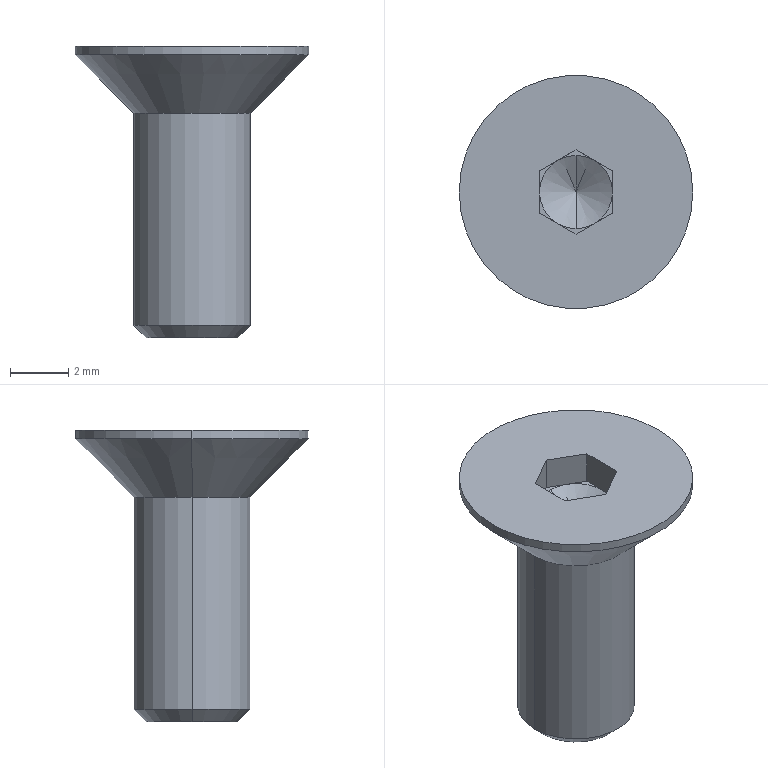Part | SolidWorks | features BaseBody 1 | 1 solid | 24 faces | box 8 x 8 x 10 mm | volume 162.002 mm3 | plane 14 | cone 6 | cylinder 4 | commonest cylinder face diameters 4 x2 8 x2
STEP:
#1=CARTESIAN_POINT('',(2.,0.,-7.271));
#2=VERTEX_POINT('',#1);
#3=CARTESIAN_POINT('',(-2.,0.,-7.271));
#4=VERTEX_POINT('',#3);
#5=CARTESIAN_POINT('',(0.,0.,-7.271));
#6=DIRECTION('',(0.,0.,1.));
#7=DIRECTION('',(1.,0.,0.));
#8=AXIS2_PLACEMENT_3D('',#5,#6,#7);
#9=CIRCLE('',#8,2.);
#10=EDGE_CURVE('',#2,#4,#9,.T.);
#11=ORIENTED_EDGE('',*,*,#10,.T.);
#12=CARTESIAN_POINT('',(-2.,0.,0.));
#13=VERTEX_POINT('',#12);
#14=CARTESIAN_POINT('',(-2.,0.,-7.7));
#15=DIRECTION('',(0.,0.,1.));
#16=VECTOR('',#15,1000.);
#17=LINE('',#14,#16);
#18=EDGE_CURVE('',#4,#13,#17,.T.);
#19=ORIENTED_EDGE('',*,*,#18,.T.);
#20=CARTESIAN_POINT('',(2.,0.,0.));
#21=VERTEX_POINT('',#20);
#22=CARTESIAN_POINT('',(0.,0.,0.));
#23=DIRECTION('',(0.,0.,-1.));
#24=DIRECTION('',(1.,0.,0.));
#25=AXIS2_PLACEMENT_3D('',#22,#23,#24);
#26=CIRCLE('',#25,2.);
#27=EDGE_CURVE('',#13,#21,#26,.T.);
#28=ORIENTED_EDGE('',*,*,#27,.T.);
#29=CARTESIAN_POINT('',(2.,0.,-7.7));
#30=DIRECTION('',(0.,0.,1.));
#31=VECTOR('',#30,1000.);
#32=LINE('',#29,#31);
#33=EDGE_CURVE('',#2,#21,#32,.T.);
#34=ORIENTED_EDGE('',*,*,#33,.F.);
#35=EDGE_LOOP('',(#11,#19,#28,#34));
#36=FACE_OUTER_BOUND('',#35,.T.);
#37=CARTESIAN_POINT('',(0.,0.,-7.7));
#38=DIRECTION('',(0.,0.,1.));
#39=DIRECTION('',(1.,0.,0.));
#40=AXIS2_PLACEMENT_3D('',#37,#38,#39);
#41=CYLINDRICAL_SURFACE('',#40,2.);
#42=ADVANCED_FACE('',(#36),#41,.T.);
#43=ORIENTED_EDGE('',*,*,#27,.F.);
#44=CARTESIAN_POINT('',(-4.,0.,2.));
#45=VERTEX_POINT('',#44);
#46=CARTESIAN_POINT('',(-4.,0.,2.));
#47=DIRECTION('',(-0.7071,0.,0.7071));
#48=VECTOR('',#47,1000.);
#49=LINE('',#46,#48);
#50=EDGE_CURVE('',#13,#45,#49,.T.);
#51=ORIENTED_EDGE('',*,*,#50,.T.);
#52=CARTESIAN_POINT('',(4.,0.,2.));
#53=VERTEX_POINT('',#52);
#54=CARTESIAN_POINT('',(0.,0.,2.));
#55=DIRECTION('',(0.,0.,-1.));
#56=DIRECTION('',(1.,0.,0.));
#57=AXIS2_PLACEMENT_3D('',#54,#55,#56);
#58=CIRCLE('',#57,4.);
#59=EDGE_CURVE('',#45,#53,#58,.T.);
#60=ORIENTED_EDGE('',*,*,#59,.T.);
#61=CARTESIAN_POINT('',(4.,0.,2.));
#62=DIRECTION('',(0.7071,0.,0.7071));
#63=VECTOR('',#62,1000.);
#64=LINE('',#61,#63);
#65=EDGE_CURVE('',#21,#53,#64,.T.);
#66=ORIENTED_EDGE('',*,*,#65,.F.);
#67=EDGE_LOOP('',(#43,#51,#60,#66));
#68=FACE_OUTER_BOUND('',#67,.T.);
#69=CARTESIAN_POINT('',(0.,0.,2.));
#70=DIRECTION('',(0.,0.,1.));
#71=DIRECTION('',(1.,0.,0.));
#72=AXIS2_PLACEMENT_3D('',#69,#70,#71);
#73=CONICAL_SURFACE('',#72,4.,0.7854);
#74=ADVANCED_FACE('',(#68),#73,.T.);
#75=CARTESIAN_POINT('',(1.571,0.,-7.7));
#76=VERTEX_POINT('',#75);
#77=CARTESIAN_POINT('',(-1.571,0.,-7.7));
#78=VERTEX_POINT('',#77);
#79=CARTESIAN_POINT('',(0.,0.,-7.7));
#80=DIRECTION('',(0.,0.,1.));
#81=DIRECTION('',(1.,0.,0.));
#82=AXIS2_PLACEMENT_3D('',#79,#80,#81);
#83=CIRCLE('',#82,1.571);
#84=EDGE_CURVE('',#76,#78,#83,.T.);
#85=ORIENTED_EDGE('',*,*,#84,.T.);
#86=CARTESIAN_POINT('',(-2.,0.,-7.27));
#87=DIRECTION('',(-0.7071,0.,0.7071));
#88=VECTOR('',#87,1000.);
#89=LINE('',#86,#88);
#90=EDGE_CURVE('',#78,#4,#89,.T.);
#91=ORIENTED_EDGE('',*,*,#90,.T.);
#92=ORIENTED_EDGE('',*,*,#10,.F.);
#93=CARTESIAN_POINT('',(2.,0.,-7.27));
#94=DIRECTION('',(0.7071,0.,0.7071));
#95=VECTOR('',#94,1000.);
#96=LINE('',#93,#95);
#97=EDGE_CURVE('',#76,#2,#96,.T.);
#98=ORIENTED_EDGE('',*,*,#97,.F.);
#99=EDGE_LOOP('',(#85,#91,#92,#98));
#100=FACE_OUTER_BOUND('',#99,.T.);
#101=CARTESIAN_POINT('',(0.,0.,-7.27));
#102=DIRECTION('',(0.,0.,1.));
#103=DIRECTION('',(1.,0.,0.));
#104=AXIS2_PLACEMENT_3D('',#101,#102,#103);
#105=CONICAL_SURFACE('',#104,2.,0.7854);
#106=ADVANCED_FACE('',(#100),#105,.T.);
#107=ORIENTED_EDGE('',*,*,#59,.F.);
#108=CARTESIAN_POINT('',(-4.,0.,2.3));
#109=VERTEX_POINT('',#108);
#110=CARTESIAN_POINT('',(-4.,0.,0.));
#111=DIRECTION('',(0.,0.,1.));
#112=VECTOR('',#111,1000.);
#113=LINE('',#110,#112);
#114=EDGE_CURVE('',#45,#109,#113,.T.);
#115=ORIENTED_EDGE('',*,*,#114,.T.);
#116=CARTESIAN_POINT('',(4.,0.,2.3));
#117=VERTEX_POINT('',#116);
#118=CARTESIAN_POINT('',(0.,0.,2.3));
#119=DIRECTION('',(0.,0.,-1.));
#120=DIRECTION('',(1.,0.,0.));
#121=AXIS2_PLACEMENT_3D('',#118,#119,#120);
#122=CIRCLE('',#121,4.);
#123=EDGE_CURVE('',#109,#117,#122,.T.);
#124=ORIENTED_EDGE('',*,*,#123,.T.);
#125=CARTESIAN_POINT('',(4.,0.,0.));
#126=DIRECTION('',(0.,0.,1.));
#127=VECTOR('',#126,1000.);
#128=LINE('',#125,#127);
#129=EDGE_CURVE('',#53,#117,#128,.T.);
#130=ORIENTED_EDGE('',*,*,#129,.F.);
#131=EDGE_LOOP('',(#107,#115,#124,#130));
#132=FACE_OUTER_BOUND('',#131,.T.);
#133=CARTESIAN_POINT('',(0.,0.,0.));
#134=DIRECTION('',(0.,0.,1.));
#135=DIRECTION('',(1.,0.,0.));
#136=AXIS2_PLACEMENT_3D('',#133,#134,#135);
#137=CYLINDRICAL_SURFACE('',#136,4.);
#138=ADVANCED_FACE('',(#132),#137,.T.);
#139=CARTESIAN_POINT('',(0.,0.,0.4283));
#140=VERTEX_POINT('',#139);
#141=CARTESIAN_POINT('',(0.,-1.25,1.15));
#142=VERTEX_POINT('',#141);
#143=CARTESIAN_POINT('',(0.,-1.25,1.15));
#144=DIRECTION('',(0.,-0.866,0.5));
#145=VECTOR('',#144,1000.);
#146=LINE('',#143,#145);
#147=EDGE_CURVE('',#140,#142,#146,.T.);
#148=ORIENTED_EDGE('',*,*,#147,.F.);
#149=CARTESIAN_POINT('',(0.,1.25,1.15));
#150=VERTEX_POINT('',#149);
#151=CARTESIAN_POINT('',(0.,1.25,1.15));
#152=DIRECTION('',(0.,0.866,0.5));
#153=VECTOR('',#152,1000.);
#154=LINE('',#151,#153);
#155=EDGE_CURVE('',#140,#150,#154,.T.);
#156=ORIENTED_EDGE('',*,*,#155,.T.);
#157=CARTESIAN_POINT('',(-0.625,1.083,1.15));
#158=VERTEX_POINT('',#157);
#159=CARTESIAN_POINT('',(0.,0.,1.15));
#160=DIRECTION('',(0.,0.,-1.));
#161=DIRECTION('',(0.,-1.,0.));
#162=AXIS2_PLACEMENT_3D('',#159,#160,#161);
#163=CIRCLE('',#162,1.25);
#164=EDGE_CURVE('',#158,#150,#163,.T.);
#165=ORIENTED_EDGE('',*,*,#164,.F.);
#166=CARTESIAN_POINT('',(-1.25,0.,1.15));
#167=VERTEX_POINT('',#166);
#168=CARTESIAN_POINT('',(0.,0.,1.15));
#169=DIRECTION('',(0.,0.,-1.));
#170=DIRECTION('',(0.,-1.,0.));
#171=AXIS2_PLACEMENT_3D('',#168,#169,#170);
#172=CIRCLE('',#171,1.25);
#173=EDGE_CURVE('',#167,#158,#172,.T.);
#174=ORIENTED_EDGE('',*,*,#173,.F.);
#175=CARTESIAN_POINT('',(-0.625,-1.083,1.15));
#176=VERTEX_POINT('',#175);
#177=CARTESIAN_POINT('',(0.,0.,1.15));
#178=DIRECTION('',(0.,0.,-1.));
#179=DIRECTION('',(0.,-1.,0.));
#180=AXIS2_PLACEMENT_3D('',#177,#178,#179);
#181=CIRCLE('',#180,1.25);
#182=EDGE_CURVE('',#176,#167,#181,.T.);
#183=ORIENTED_EDGE('',*,*,#182,.F.);
#184=CARTESIAN_POINT('',(0.,0.,1.15));
#185=DIRECTION('',(0.,0.,-1.));
#186=DIRECTION('',(0.,-1.,0.));
#187=AXIS2_PLACEMENT_3D('',#184,#185,#186);
#188=CIRCLE('',#187,1.25);
#189=EDGE_CURVE('',#142,#176,#188,.T.);
#190=ORIENTED_EDGE('',*,*,#189,.F.);
#191=EDGE_LOOP('',(#148,#156,#165,#174,#183,#190));
#192=FACE_OUTER_BOUND('',#191,.T.);
#193=CARTESIAN_POINT('',(0.,0.,1.15));
#194=DIRECTION('',(0.,0.,1.));
#195=DIRECTION('',(0.,-1.,0.));
#196=AXIS2_PLACEMENT_3D('',#193,#194,#195);
#197=CONICAL_SURFACE('',#196,1.25,1.047);
#198=ADVANCED_FACE('',(#192),#197,.F.);
#199=ORIENTED_EDGE('',*,*,#18,.F.);
#200=CARTESIAN_POINT('',(0.,0.,-7.271));
#201=DIRECTION('',(0.,0.,1.));
#202=DIRECTION('',(1.,0.,0.));
#203=AXIS2_PLACEMENT_3D('',#200,#201,#202);
#204=CIRCLE('',#203,2.);
#205=EDGE_CURVE('',#4,#2,#204,.T.);
#206=ORIENTED_EDGE('',*,*,#205,.T.);
#207=ORIENTED_EDGE('',*,*,#33,.T.);
#208=CARTESIAN_POINT('',(0.,0.,0.));
#209=DIRECTION('',(0.,0.,-1.));
#210=DIRECTION('',(1.,0.,0.));
#211=AXIS2_PLACEMENT_3D('',#208,#209,#210);
#212=CIRCLE('',#211,2.);
#213=EDGE_CURVE('',#21,#13,#212,.T.);
#214=ORIENTED_EDGE('',*,*,#213,.T.);
#215=EDGE_LOOP('',(#199,#206,#207,#214));
#216=FACE_OUTER_BOUND('',#215,.T.);
#217=CARTESIAN_POINT('',(0.,0.,-7.7));
#218=DIRECTION('',(0.,0.,1.));
#219=DIRECTION('',(1.,0.,0.));
#220=AXIS2_PLACEMENT_3D('',#217,#218,#219);
#221=CYLINDRICAL_SURFACE('',#220,2.);
#222=ADVANCED_FACE('',(#216),#221,.T.);
#223=ORIENTED_EDGE('',*,*,#50,.F.);
#224=ORIENTED_EDGE('',*,*,#213,.F.);
#225=ORIENTED_EDGE('',*,*,#65,.T.);
#226=CARTESIAN_POINT('',(0.,0.,2.));
#227=DIRECTION('',(0.,0.,-1.));
#228=DIRECTION('',(1.,0.,0.));
#229=AXIS2_PLACEMENT_3D('',#226,#227,#228);
#230=CIRCLE('',#229,4.);
#231=EDGE_CURVE('',#53,#45,#230,.T.);
#232=ORIENTED_EDGE('',*,*,#231,.T.);
#233=EDGE_LOOP('',(#223,#224,#225,#232));
#234=FACE_OUTER_BOUND('',#233,.T.);
#235=CARTESIAN_POINT('',(0.,0.,2.));
#236=DIRECTION('',(0.,0.,1.));
#237=DIRECTION('',(1.,0.,0.));
#238=AXIS2_PLACEMENT_3D('',#235,#236,#237);
#239=CONICAL_SURFACE('',#238,4.,0.7854);
#240=ADVANCED_FACE('',(#234),#239,.T.);
#241=ORIENTED_EDGE('',*,*,#90,.F.);
#242=CARTESIAN_POINT('',(0.,0.,-7.7));
#243=DIRECTION('',(0.,0.,1.));
#244=DIRECTION('',(1.,0.,0.));
#245=AXIS2_PLACEMENT_3D('',#242,#243,#244);
#246=CIRCLE('',#245,1.571);
#247=EDGE_CURVE('',#78,#76,#246,.T.);
#248=ORIENTED_EDGE('',*,*,#247,.T.);
#249=ORIENTED_EDGE('',*,*,#97,.T.);
#250=ORIENTED_EDGE('',*,*,#205,.F.);
#251=EDGE_LOOP('',(#241,#248,#249,#250));
#252=FACE_OUTER_BOUND('',#251,.T.);
#253=CARTESIAN_POINT('',(0.,0.,-7.27));
#254=DIRECTION('',(0.,0.,1.));
#255=DIRECTION('',(1.,0.,0.));
#256=AXIS2_PLACEMENT_3D('',#253,#254,#255);
#257=CONICAL_SURFACE('',#256,2.,0.7854);
#258=ADVANCED_FACE('',(#252),#257,.T.);
#259=ORIENTED_EDGE('',*,*,#114,.F.);
#260=ORIENTED_EDGE('',*,*,#231,.F.);
#261=ORIENTED_EDGE('',*,*,#129,.T.);
#262=CARTESIAN_POINT('',(0.,0.,2.3));
#263=DIRECTION('',(0.,0.,-1.));
#264=DIRECTION('',(1.,0.,0.));
#265=AXIS2_PLACEMENT_3D('',#262,#263,#264);
#266=CIRCLE('',#265,4.);
#267=EDGE_CURVE('',#117,#109,#266,.T.);
#268=ORIENTED_EDGE('',*,*,#267,.T.);
#269=EDGE_LOOP('',(#259,#260,#261,#268));
#270=FACE_OUTER_BOUND('',#269,.T.);
#271=CARTESIAN_POINT('',(0.,0.,0.));
#272=DIRECTION('',(0.,0.,1.));
#273=DIRECTION('',(1.,0.,0.));
#274=AXIS2_PLACEMENT_3D('',#271,#272,#273);
#275=CYLINDRICAL_SURFACE('',#274,4.);
#276=ADVANCED_FACE('',(#270),#275,.T.);
#277=ORIENTED_EDGE('',*,*,#84,.F.);
#278=ORIENTED_EDGE('',*,*,#247,.F.);
#279=EDGE_LOOP('',(#277,#278));
#280=FACE_OUTER_BOUND('',#279,.T.);
#281=CARTESIAN_POINT('',(0.,1.571,-7.7));
#282=DIRECTION('',(0.,0.,1.));
#283=DIRECTION('',(1.,0.,0.));
#284=AXIS2_PLACEMENT_3D('',#281,#282,#283);
#285=PLANE('',#284);
#286=ADVANCED_FACE('',(#280),#285,.F.);
#287=CARTESIAN_POINT('',(-1.25,-0.7217,2.3));
#288=VERTEX_POINT('',#287);
#289=CARTESIAN_POINT('',(0.,-1.443,2.3));
#290=VERTEX_POINT('',#289);
#291=CARTESIAN_POINT('',(-1.25,-0.7217,2.3));
#292=DIRECTION('',(0.866,-0.5,0.));
#293=VECTOR('',#292,1000.);
#294=LINE('',#291,#293);
#295=EDGE_CURVE('',#288,#290,#294,.T.);
#296=ORIENTED_EDGE('',*,*,#295,.F.);
#297=CARTESIAN_POINT('',(-1.25,0.7217,2.3));
#298=VERTEX_POINT('',#297);
#299=CARTESIAN_POINT('',(-1.25,0.,2.3));
#300=DIRECTION('',(0.,-1.,0.));
#301=VECTOR('',#300,1000.);
#302=LINE('',#299,#301);
#303=EDGE_CURVE('',#298,#288,#302,.T.);
#304=ORIENTED_EDGE('',*,*,#303,.F.);
#305=CARTESIAN_POINT('',(0.,1.443,2.3));
#306=VERTEX_POINT('',#305);
#307=CARTESIAN_POINT('',(0.,1.443,2.3));
#308=DIRECTION('',(-0.866,-0.5,0.));
#309=VECTOR('',#308,1000.);
#310=LINE('',#307,#309);
#311=EDGE_CURVE('',#306,#298,#310,.T.);
#312=ORIENTED_EDGE('',*,*,#311,.F.);
#313=CARTESIAN_POINT('',(1.25,0.7217,2.3));
#314=VERTEX_POINT('',#313);
#315=CARTESIAN_POINT('',(1.25,0.7217,2.3));
#316=DIRECTION('',(-0.866,0.5,0.));
#317=VECTOR('',#316,1000.);
#318=LINE('',#315,#317);
#319=EDGE_CURVE('',#314,#306,#318,.T.);
#320=ORIENTED_EDGE('',*,*,#319,.F.);
#321=CARTESIAN_POINT('',(1.25,-0.7217,2.3));
#322=VERTEX_POINT('',#321);
#323=CARTESIAN_POINT('',(1.25,0.,2.3));
#324=DIRECTION('',(0.,1.,0.));
#325=VECTOR('',#324,1000.);
#326=LINE('',#323,#325);
#327=EDGE_CURVE('',#322,#314,#326,.T.);
#328=ORIENTED_EDGE('',*,*,#327,.F.);
#329=CARTESIAN_POINT('',(0.,-1.443,2.3));
#330=DIRECTION('',(0.866,0.5,0.));
#331=VECTOR('',#330,1000.);
#332=LINE('',#329,#331);
#333=EDGE_CURVE('',#290,#322,#332,.T.);
#334=ORIENTED_EDGE('',*,*,#333,.F.);
#335=EDGE_LOOP('',(#296,#304,#312,#320,#328,#334));
#336=FACE_BOUND('',#335,.T.);
#337=ORIENTED_EDGE('',*,*,#267,.F.);
#338=ORIENTED_EDGE('',*,*,#123,.F.);
#339=EDGE_LOOP('',(#337,#338));
#340=FACE_OUTER_BOUND('',#339,.T.);
#341=CARTESIAN_POINT('',(0.,0.,2.3));
#342=DIRECTION('',(0.,0.,-1.));
#343=DIRECTION('',(-1.,0.,0.));
#344=AXIS2_PLACEMENT_3D('',#341,#342,#343);
#345=PLANE('',#344);
#346=ADVANCED_FACE('',(#336,#340),#345,.F.);
#347=CARTESIAN_POINT('',(1.25,-0.7217,1.15));
#348=VERTEX_POINT('',#347);
#349=CARTESIAN_POINT('',(1.25,-0.7217,1.15));
#350=DIRECTION('',(0.,0.,1.));
#351=VECTOR('',#350,1000.);
#352=LINE('',#349,#351);
#353=EDGE_CURVE('',#348,#322,#352,.T.);
#354=ORIENTED_EDGE('',*,*,#353,.F.);
#355=CARTESIAN_POINT('',(0.625,-1.083,1.15));
#356=VERTEX_POINT('',#355);
#357=CARTESIAN_POINT('',(0.,-1.443,1.15));
#358=DIRECTION('',(0.866,0.5,0.));
#359=VECTOR('',#358,1000.);
#360=LINE('',#357,#359);
#361=EDGE_CURVE('',#356,#348,#360,.T.);
#362=ORIENTED_EDGE('',*,*,#361,.F.);
#363=CARTESIAN_POINT('',(0.,-1.443,1.15));
#364=VERTEX_POINT('',#363);
#365=CARTESIAN_POINT('',(0.,-1.443,1.15));
#366=DIRECTION('',(0.866,0.5,0.));
#367=VECTOR('',#366,1000.);
#368=LINE('',#365,#367);
#369=EDGE_CURVE('',#364,#356,#368,.T.);
#370=ORIENTED_EDGE('',*,*,#369,.F.);
#371=CARTESIAN_POINT('',(0.,-1.443,1.15));
#372=DIRECTION('',(0.,0.,-1.));
#373=VECTOR('',#372,1000.);
#374=LINE('',#371,#373);
#375=EDGE_CURVE('',#290,#364,#374,.T.);
#376=ORIENTED_EDGE('',*,*,#375,.F.);
#377=ORIENTED_EDGE('',*,*,#333,.T.);
#378=EDGE_LOOP('',(#354,#362,#370,#376,#377));
#379=FACE_OUTER_BOUND('',#378,.T.);
#380=CARTESIAN_POINT('',(0.,-1.443,1.15));
#381=DIRECTION('',(0.5,-0.866,0.));
#382=DIRECTION('',(0.866,0.5,0.));
#383=AXIS2_PLACEMENT_3D('',#380,#381,#382);
#384=PLANE('',#383);
#385=ADVANCED_FACE('',(#379),#384,.F.);
#386=ORIENTED_EDGE('',*,*,#375,.T.);
#387=CARTESIAN_POINT('',(-1.25,-0.7217,1.15));
#388=DIRECTION('',(0.866,-0.5,0.));
#389=VECTOR('',#388,1000.);
#390=LINE('',#387,#389);
#391=EDGE_CURVE('',#176,#364,#390,.T.);
#392=ORIENTED_EDGE('',*,*,#391,.F.);
#393=CARTESIAN_POINT('',(-1.25,-0.7217,1.15));
#394=VERTEX_POINT('',#393);
#395=CARTESIAN_POINT('',(-1.25,-0.7217,1.15));
#396=DIRECTION('',(0.866,-0.5,0.));
#397=VECTOR('',#396,1000.);
#398=LINE('',#395,#397);
#399=EDGE_CURVE('',#394,#176,#398,.T.);
#400=ORIENTED_EDGE('',*,*,#399,.F.);
#401=CARTESIAN_POINT('',(-1.25,-0.7217,1.15));
#402=DIRECTION('',(0.,0.,-1.));
#403=VECTOR('',#402,1000.);
#404=LINE('',#401,#403);
#405=EDGE_CURVE('',#288,#394,#404,.T.);
#406=ORIENTED_EDGE('',*,*,#405,.F.);
#407=ORIENTED_EDGE('',*,*,#295,.T.);
#408=EDGE_LOOP('',(#386,#392,#400,#406,#407));
#409=FACE_OUTER_BOUND('',#408,.T.);
#410=CARTESIAN_POINT('',(-1.25,-0.7217,1.15));
#411=DIRECTION('',(-0.5,-0.866,0.));
#412=DIRECTION('',(0.866,-0.5,0.));
#413=AXIS2_PLACEMENT_3D('',#410,#411,#412);
#414=PLANE('',#413);
#415=ADVANCED_FACE('',(#409),#414,.F.);
#416=ORIENTED_EDGE('',*,*,#405,.T.);
#417=CARTESIAN_POINT('',(-1.25,0.7217,1.15));
#418=DIRECTION('',(0.,-1.,0.));
#419=VECTOR('',#418,1000.);
#420=LINE('',#417,#419);
#421=EDGE_CURVE('',#167,#394,#420,.T.);
#422=ORIENTED_EDGE('',*,*,#421,.F.);
#423=CARTESIAN_POINT('',(-1.25,0.7217,1.15));
#424=VERTEX_POINT('',#423);
#425=CARTESIAN_POINT('',(-1.25,0.7217,1.15));
#426=DIRECTION('',(0.,-1.,0.));
#427=VECTOR('',#426,1000.);
#428=LINE('',#425,#427);
#429=EDGE_CURVE('',#424,#167,#428,.T.);
#430=ORIENTED_EDGE('',*,*,#429,.F.);
#431=CARTESIAN_POINT('',(-1.25,0.7217,1.15));
#432=DIRECTION('',(0.,0.,-1.));
#433=VECTOR('',#432,1000.);
#434=LINE('',#431,#433);
#435=EDGE_CURVE('',#298,#424,#434,.T.);
#436=ORIENTED_EDGE('',*,*,#435,.F.);
#437=ORIENTED_EDGE('',*,*,#303,.T.);
#438=EDGE_LOOP('',(#416,#422,#430,#436,#437));
#439=FACE_OUTER_BOUND('',#438,.T.);
#440=CARTESIAN_POINT('',(-1.25,0.7217,1.15));
#441=DIRECTION('',(-1.,0.,0.));
#442=DIRECTION('',(0.,0.,1.));
#443=AXIS2_PLACEMENT_3D('',#440,#441,#442);
#444=PLANE('',#443);
#445=ADVANCED_FACE('',(#439),#444,.F.);
#446=ORIENTED_EDGE('',*,*,#435,.T.);
#447=CARTESIAN_POINT('',(0.,1.443,1.15));
#448=DIRECTION('',(-0.866,-0.5,0.));
#449=VECTOR('',#448,1000.);
#450=LINE('',#447,#449);
#451=EDGE_CURVE('',#158,#424,#450,.T.);
#452=ORIENTED_EDGE('',*,*,#451,.F.);
#453=CARTESIAN_POINT('',(0.,1.443,1.15));
#454=VERTEX_POINT('',#453);
#455=CARTESIAN_POINT('',(0.,1.443,1.15));
#456=DIRECTION('',(-0.866,-0.5,0.));
#457=VECTOR('',#456,1000.);
#458=LINE('',#455,#457);
#459=EDGE_CURVE('',#454,#158,#458,.T.);
#460=ORIENTED_EDGE('',*,*,#459,.F.);
#461=CARTESIAN_POINT('',(0.,1.443,1.15));
#462=DIRECTION('',(0.,0.,-1.));
#463=VECTOR('',#462,1000.);
#464=LINE('',#461,#463);
#465=EDGE_CURVE('',#306,#454,#464,.T.);
#466=ORIENTED_EDGE('',*,*,#465,.F.);
#467=ORIENTED_EDGE('',*,*,#311,.T.);
#468=EDGE_LOOP('',(#446,#452,#460,#466,#467));
#469=FACE_OUTER_BOUND('',#468,.T.);
#470=CARTESIAN_POINT('',(0.,1.443,1.15));
#471=DIRECTION('',(-0.5,0.866,0.));
#472=DIRECTION('',(-0.866,-0.5,0.));
#473=AXIS2_PLACEMENT_3D('',#470,#471,#472);
#474=PLANE('',#473);
#475=ADVANCED_FACE('',(#469),#474,.F.);
#476=ORIENTED_EDGE('',*,*,#465,.T.);
#477=CARTESIAN_POINT('',(0.625,1.083,1.15));
#478=VERTEX_POINT('',#477);
#479=CARTESIAN_POINT('',(1.25,0.7217,1.15));
#480=DIRECTION('',(-0.866,0.5,0.));
#481=VECTOR('',#480,1000.);
#482=LINE('',#479,#481);
#483=EDGE_CURVE('',#478,#454,#482,.T.);
#484=ORIENTED_EDGE('',*,*,#483,.F.);
#485=CARTESIAN_POINT('',(1.25,0.7217,1.15));
#486=VERTEX_POINT('',#485);
#487=CARTESIAN_POINT('',(1.25,0.7217,1.15));
#488=DIRECTION('',(-0.866,0.5,0.));
#489=VECTOR('',#488,1000.);
#490=LINE('',#487,#489);
#491=EDGE_CURVE('',#486,#478,#490,.T.);
#492=ORIENTED_EDGE('',*,*,#491,.F.);
#493=CARTESIAN_POINT('',(1.25,0.7217,1.15));
#494=DIRECTION('',(0.,0.,-1.));
#495=VECTOR('',#494,1000.);
#496=LINE('',#493,#495);
#497=EDGE_CURVE('',#314,#486,#496,.T.);
#498=ORIENTED_EDGE('',*,*,#497,.F.);
#499=ORIENTED_EDGE('',*,*,#319,.T.);
#500=EDGE_LOOP('',(#476,#484,#492,#498,#499));
#501=FACE_OUTER_BOUND('',#500,.T.);
#502=CARTESIAN_POINT('',(1.25,0.7217,1.15));
#503=DIRECTION('',(0.5,0.866,0.));
#504=DIRECTION('',(-0.866,0.5,0.));
#505=AXIS2_PLACEMENT_3D('',#502,#503,#504);
#506=PLANE('',#505);
#507=ADVANCED_FACE('',(#501),#506,.F.);
#508=ORIENTED_EDGE('',*,*,#497,.T.);
#509=CARTESIAN_POINT('',(1.25,0.,1.15));
#510=VERTEX_POINT('',#509);
#511=CARTESIAN_POINT('',(1.25,-0.7217,1.15));
#512=DIRECTION('',(0.,1.,0.));
#513=VECTOR('',#512,1000.);
#514=LINE('',#511,#513);
#515=EDGE_CURVE('',#510,#486,#514,.T.);
#516=ORIENTED_EDGE('',*,*,#515,.F.);
#517=CARTESIAN_POINT('',(1.25,-0.7217,1.15));
#518=DIRECTION('',(0.,1.,0.));
#519=VECTOR('',#518,1000.);
#520=LINE('',#517,#519);
#521=EDGE_CURVE('',#348,#510,#520,.T.);
#522=ORIENTED_EDGE('',*,*,#521,.F.);
#523=ORIENTED_EDGE('',*,*,#353,.T.);
#524=ORIENTED_EDGE('',*,*,#327,.T.);
#525=EDGE_LOOP('',(#508,#516,#522,#523,#524));
#526=FACE_OUTER_BOUND('',#525,.T.);
#527=CARTESIAN_POINT('',(1.25,-0.7217,1.15));
#528=DIRECTION('',(1.,0.,0.));
#529=DIRECTION('',(0.,0.,-1.));
#530=AXIS2_PLACEMENT_3D('',#527,#528,#529);
#531=PLANE('',#530);
#532=ADVANCED_FACE('',(#526),#531,.F.);
#533=CARTESIAN_POINT('',(0.,0.,1.15));
#534=DIRECTION('',(0.,0.,-1.));
#535=DIRECTION('',(0.,-1.,0.));
#536=AXIS2_PLACEMENT_3D('',#533,#534,#535);
#537=CIRCLE('',#536,1.25);
#538=EDGE_CURVE('',#510,#356,#537,.T.);
#539=ORIENTED_EDGE('',*,*,#538,.T.);
#540=ORIENTED_EDGE('',*,*,#361,.T.);
#541=ORIENTED_EDGE('',*,*,#521,.T.);
#542=EDGE_LOOP('',(#539,#540,#541));
#543=FACE_OUTER_BOUND('',#542,.T.);
#544=CARTESIAN_POINT('',(0.,0.,1.15));
#545=DIRECTION('',(0.,0.,1.));
#546=DIRECTION('',(1.,0.,0.));
#547=AXIS2_PLACEMENT_3D('',#544,#545,#546);
#548=PLANE('',#547);
#549=ADVANCED_FACE('',(#543),#548,.T.);
#550=CARTESIAN_POINT('',(0.,0.,1.15));
#551=DIRECTION('',(0.,0.,-1.));
#552=DIRECTION('',(0.,-1.,0.));
#553=AXIS2_PLACEMENT_3D('',#550,#551,#552);
#554=CIRCLE('',#553,1.25);
#555=EDGE_CURVE('',#356,#142,#554,.T.);
#556=ORIENTED_EDGE('',*,*,#555,.T.);
#557=ORIENTED_EDGE('',*,*,#189,.T.);
#558=ORIENTED_EDGE('',*,*,#391,.T.);
#559=ORIENTED_EDGE('',*,*,#369,.T.);
#560=EDGE_LOOP('',(#556,#557,#558,#559));
#561=FACE_OUTER_BOUND('',#560,.T.);
#562=CARTESIAN_POINT('',(0.,0.,1.15));
#563=DIRECTION('',(0.,0.,1.));
#564=DIRECTION('',(1.,0.,0.));
#565=AXIS2_PLACEMENT_3D('',#562,#563,#564);
#566=PLANE('',#565);
#567=ADVANCED_FACE('',(#561),#566,.T.);
#568=ORIENTED_EDGE('',*,*,#182,.T.);
#569=ORIENTED_EDGE('',*,*,#421,.T.);
#570=ORIENTED_EDGE('',*,*,#399,.T.);
#571=EDGE_LOOP('',(#568,#569,#570));
#572=FACE_OUTER_BOUND('',#571,.T.);
#573=CARTESIAN_POINT('',(0.,0.,1.15));
#574=DIRECTION('',(0.,0.,1.));
#575=DIRECTION('',(1.,0.,0.));
#576=AXIS2_PLACEMENT_3D('',#573,#574,#575);
#577=PLANE('',#576);
#578=ADVANCED_FACE('',(#572),#577,.T.);
#579=ORIENTED_EDGE('',*,*,#173,.T.);
#580=ORIENTED_EDGE('',*,*,#451,.T.);
#581=ORIENTED_EDGE('',*,*,#429,.T.);
#582=EDGE_LOOP('',(#579,#580,#581));
#583=FACE_OUTER_BOUND('',#582,.T.);
#584=CARTESIAN_POINT('',(0.,0.,1.15));
#585=DIRECTION('',(0.,0.,1.));
#586=DIRECTION('',(1.,0.,0.));
#587=AXIS2_PLACEMENT_3D('',#584,#585,#586);
#588=PLANE('',#587);
#589=ADVANCED_FACE('',(#583),#588,.T.);
#590=ORIENTED_EDGE('',*,*,#164,.T.);
#591=CARTESIAN_POINT('',(0.,0.,1.15));
#592=DIRECTION('',(0.,0.,-1.));
#593=DIRECTION('',(0.,-1.,0.));
#594=AXIS2_PLACEMENT_3D('',#591,#592,#593);
#595=CIRCLE('',#594,1.25);
#596=EDGE_CURVE('',#150,#478,#595,.T.);
#597=ORIENTED_EDGE('',*,*,#596,.T.);
#598=ORIENTED_EDGE('',*,*,#483,.T.);
#599=ORIENTED_EDGE('',*,*,#459,.T.);
#600=EDGE_LOOP('',(#590,#597,#598,#599));
#601=FACE_OUTER_BOUND('',#600,.T.);
#602=CARTESIAN_POINT('',(0.,0.,1.15));
#603=DIRECTION('',(0.,0.,1.));
#604=DIRECTION('',(1.,0.,0.));
#605=AXIS2_PLACEMENT_3D('',#602,#603,#604);
#606=PLANE('',#605);
#607=ADVANCED_FACE('',(#601),#606,.T.);
#608=CARTESIAN_POINT('',(0.,0.,1.15));
#609=DIRECTION('',(0.,0.,-1.));
#610=DIRECTION('',(0.,-1.,0.));
#611=AXIS2_PLACEMENT_3D('',#608,#609,#610);
#612=CIRCLE('',#611,1.25);
#613=EDGE_CURVE('',#478,#510,#612,.T.);
#614=ORIENTED_EDGE('',*,*,#613,.T.);
#615=ORIENTED_EDGE('',*,*,#515,.T.);
#616=ORIENTED_EDGE('',*,*,#491,.T.);
#617=EDGE_LOOP('',(#614,#615,#616));
#618=FACE_OUTER_BOUND('',#617,.T.);
#619=CARTESIAN_POINT('',(0.,0.,1.15));
#620=DIRECTION('',(0.,0.,1.));
#621=DIRECTION('',(1.,0.,0.));
#622=AXIS2_PLACEMENT_3D('',#619,#620,#621);
#623=PLANE('',#622);
#624=ADVANCED_FACE('',(#618),#623,.T.);
#625=ORIENTED_EDGE('',*,*,#155,.F.);
#626=ORIENTED_EDGE('',*,*,#147,.T.);
#627=ORIENTED_EDGE('',*,*,#555,.F.);
#628=ORIENTED_EDGE('',*,*,#538,.F.);
#629=ORIENTED_EDGE('',*,*,#613,.F.);
#630=ORIENTED_EDGE('',*,*,#596,.F.);
#631=EDGE_LOOP('',(#625,#626,#627,#628,#629,#630));
#632=FACE_OUTER_BOUND('',#631,.T.);
#633=CARTESIAN_POINT('',(0.,0.,1.15));
#634=DIRECTION('',(0.,0.,1.));
#635=DIRECTION('',(0.,-1.,0.));
#636=AXIS2_PLACEMENT_3D('',#633,#634,#635);
#637=CONICAL_SURFACE('',#636,1.25,1.047);
#638=ADVANCED_FACE('',(#632),#637,.F.);
#639=CLOSED_SHELL('',(#42,#74,#106,#138,#198,#222,#240,#258,#276,#286,#346,#385,#415,#445,#475,#507,#532,#549,#567,#578,#589,#607,#624,#638));
#640=MANIFOLD_SOLID_BREP('',#639);
#641=CARTESIAN_POINT('',(0.,0.,0.));
#642=DIRECTION('',(0.,0.,1.));
#643=DIRECTION('',(1.,0.,0.));
#644=AXIS2_PLACEMENT_3D('',#641,#642,#643);
#645=(LENGTH_UNIT()NAMED_UNIT(*)SI_UNIT(.MILLI.,.METRE.));
#646=UNCERTAINTY_MEASURE_WITH_UNIT(LENGTH_MEASURE(0.00001),#645,'','');
#647=(NAMED_UNIT(*)PLANE_ANGLE_UNIT()SI_UNIT($,.RADIAN.));
#648=(NAMED_UNIT(*)SI_UNIT($,.STERADIAN.)SOLID_ANGLE_UNIT());
#649=(GEOMETRIC_REPRESENTATION_CONTEXT(3)GLOBAL_UNCERTAINTY_ASSIGNED_CONTEXT((#646))GLOBAL_UNIT_ASSIGNED_CONTEXT((#645,#647,#648))REPRESENTATION_CONTEXT('',''));
#650=ADVANCED_BREP_SHAPE_REPRESENTATION('',(#640,#644),#649);